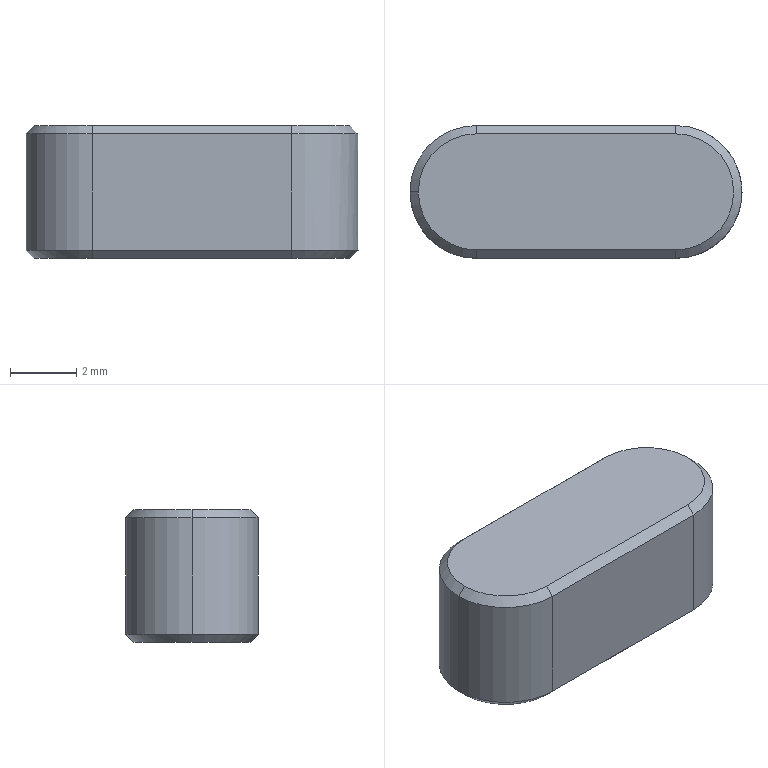Part | SolidWorks | features Boss 2, Chamfer 1, Extrusion 1 | 1 solid | 17 faces | box 10 x 4 x 4 mm | volume 144.763 mm3 | plane 8 | cone 6 | cylinder 3 | commonest cylinder face diameters 4 x3
STEP:
#1=CARTESIAN_POINT('',(-7.75,0.,2.));
#2=VERTEX_POINT('',#1);
#3=CARTESIAN_POINT('',(-6.,-1.75,2.));
#4=VERTEX_POINT('',#3);
#5=CARTESIAN_POINT('',(-6.,0.,2.));
#6=DIRECTION('',(0.,0.,1.));
#7=DIRECTION('',(-1.,0.,0.));
#8=AXIS2_PLACEMENT_3D('',#5,#6,#7);
#9=CIRCLE('',#8,1.75);
#10=EDGE_CURVE('',#2,#4,#9,.T.);
#11=ORIENTED_EDGE('',*,*,#10,.F.);
#12=CARTESIAN_POINT('',(-8.,0.,1.75));
#13=VERTEX_POINT('',#12);
#14=CARTESIAN_POINT('',(-7.75,0.,2.));
#15=DIRECTION('',(-0.7071,0.,-0.7071));
#16=VECTOR('',#15,1000.);
#17=LINE('',#14,#16);
#18=EDGE_CURVE('',#2,#13,#17,.T.);
#19=ORIENTED_EDGE('',*,*,#18,.T.);
#20=CARTESIAN_POINT('',(-6.,-2.,1.75));
#21=VERTEX_POINT('',#20);
#22=CARTESIAN_POINT('',(-6.,0.,1.75));
#23=DIRECTION('',(0.,0.,-1.));
#24=DIRECTION('',(-1.,0.,0.));
#25=AXIS2_PLACEMENT_3D('',#22,#23,#24);
#26=CIRCLE('',#25,2.);
#27=EDGE_CURVE('',#21,#13,#26,.T.);
#28=ORIENTED_EDGE('',*,*,#27,.F.);
#29=CARTESIAN_POINT('',(-6.,-1.75,2.));
#30=DIRECTION('',(0.,-0.7071,-0.7071));
#31=VECTOR('',#30,1000.);
#32=LINE('',#29,#31);
#33=EDGE_CURVE('',#4,#21,#32,.T.);
#34=ORIENTED_EDGE('',*,*,#33,.F.);
#35=EDGE_LOOP('',(#11,#19,#28,#34));
#36=FACE_OUTER_BOUND('',#35,.T.);
#37=CARTESIAN_POINT('',(-6.,0.,2.));
#38=DIRECTION('',(0.,0.,-1.));
#39=DIRECTION('',(-1.,0.,0.));
#40=AXIS2_PLACEMENT_3D('',#37,#38,#39);
#41=CONICAL_SURFACE('',#40,1.75,0.7854);
#42=ADVANCED_FACE('',(#36),#41,.T.);
#43=CARTESIAN_POINT('',(1.75,0.,-2.));
#44=VERTEX_POINT('',#43);
#45=CARTESIAN_POINT('',(0.,-1.75,-2.));
#46=VERTEX_POINT('',#45);
#47=CARTESIAN_POINT('',(0.,0.,-2.));
#48=DIRECTION('',(0.,0.,-1.));
#49=DIRECTION('',(-1.,0.,0.));
#50=AXIS2_PLACEMENT_3D('',#47,#48,#49);
#51=CIRCLE('',#50,1.75);
#52=EDGE_CURVE('',#44,#46,#51,.T.);
#53=ORIENTED_EDGE('',*,*,#52,.F.);
#54=CARTESIAN_POINT('',(2.,0.,-1.75));
#55=VERTEX_POINT('',#54);
#56=CARTESIAN_POINT('',(2.,0.,-1.75));
#57=DIRECTION('',(0.7071,0.,0.7071));
#58=VECTOR('',#57,1000.);
#59=LINE('',#56,#58);
#60=EDGE_CURVE('',#44,#55,#59,.T.);
#61=ORIENTED_EDGE('',*,*,#60,.T.);
#62=CARTESIAN_POINT('',(0.,-2.,-1.75));
#63=VERTEX_POINT('',#62);
#64=CARTESIAN_POINT('',(0.,0.,-1.75));
#65=DIRECTION('',(0.,0.,1.));
#66=DIRECTION('',(-1.,0.,0.));
#67=AXIS2_PLACEMENT_3D('',#64,#65,#66);
#68=CIRCLE('',#67,2.);
#69=EDGE_CURVE('',#63,#55,#68,.T.);
#70=ORIENTED_EDGE('',*,*,#69,.F.);
#71=CARTESIAN_POINT('',(0.,-1.75,-2.));
#72=DIRECTION('',(0.,-0.7071,0.7071));
#73=VECTOR('',#72,1000.);
#74=LINE('',#71,#73);
#75=EDGE_CURVE('',#46,#63,#74,.T.);
#76=ORIENTED_EDGE('',*,*,#75,.F.);
#77=EDGE_LOOP('',(#53,#61,#70,#76));
#78=FACE_OUTER_BOUND('',#77,.T.);
#79=CARTESIAN_POINT('',(0.,0.,-1.75));
#80=DIRECTION('',(0.,0.,1.));
#81=DIRECTION('',(1.,0.,0.));
#82=AXIS2_PLACEMENT_3D('',#79,#80,#81);
#83=CONICAL_SURFACE('',#82,2.,0.7854);
#84=ADVANCED_FACE('',(#78),#83,.T.);
#85=ORIENTED_EDGE('',*,*,#27,.T.);
#86=CARTESIAN_POINT('',(-8.,0.,-1.75));
#87=VERTEX_POINT('',#86);
#88=CARTESIAN_POINT('',(-8.,0.,2.));
#89=DIRECTION('',(0.,0.,-1.));
#90=VECTOR('',#89,1000.);
#91=LINE('',#88,#90);
#92=EDGE_CURVE('',#13,#87,#91,.T.);
#93=ORIENTED_EDGE('',*,*,#92,.T.);
#94=CARTESIAN_POINT('',(-6.,-2.,-1.75));
#95=VERTEX_POINT('',#94);
#96=CARTESIAN_POINT('',(-6.,0.,-1.75));
#97=DIRECTION('',(0.,0.,1.));
#98=DIRECTION('',(-1.,0.,0.));
#99=AXIS2_PLACEMENT_3D('',#96,#97,#98);
#100=CIRCLE('',#99,2.);
#101=EDGE_CURVE('',#87,#95,#100,.T.);
#102=ORIENTED_EDGE('',*,*,#101,.T.);
#103=CARTESIAN_POINT('',(-6.,-2.,2.));
#104=DIRECTION('',(0.,0.,-1.));
#105=VECTOR('',#104,1000.);
#106=LINE('',#103,#105);
#107=EDGE_CURVE('',#21,#95,#106,.T.);
#108=ORIENTED_EDGE('',*,*,#107,.F.);
#109=EDGE_LOOP('',(#85,#93,#102,#108));
#110=FACE_OUTER_BOUND('',#109,.T.);
#111=CARTESIAN_POINT('',(-6.,0.,2.));
#112=DIRECTION('',(0.,0.,-1.));
#113=DIRECTION('',(-1.,0.,0.));
#114=AXIS2_PLACEMENT_3D('',#111,#112,#113);
#115=CYLINDRICAL_SURFACE('',#114,2.);
#116=ADVANCED_FACE('',(#110),#115,.T.);
#117=ORIENTED_EDGE('',*,*,#92,.F.);
#118=CARTESIAN_POINT('',(-6.,2.,1.75));
#119=VERTEX_POINT('',#118);
#120=CARTESIAN_POINT('',(-6.,0.,1.75));
#121=DIRECTION('',(0.,0.,-1.));
#122=DIRECTION('',(-1.,0.,0.));
#123=AXIS2_PLACEMENT_3D('',#120,#121,#122);
#124=CIRCLE('',#123,2.);
#125=EDGE_CURVE('',#13,#119,#124,.T.);
#126=ORIENTED_EDGE('',*,*,#125,.T.);
#127=CARTESIAN_POINT('',(-6.,2.,-1.75));
#128=VERTEX_POINT('',#127);
#129=CARTESIAN_POINT('',(-6.,2.,2.));
#130=DIRECTION('',(0.,0.,-1.));
#131=VECTOR('',#130,1000.);
#132=LINE('',#129,#131);
#133=EDGE_CURVE('',#119,#128,#132,.T.);
#134=ORIENTED_EDGE('',*,*,#133,.T.);
#135=CARTESIAN_POINT('',(-6.,0.,-1.75));
#136=DIRECTION('',(0.,0.,1.));
#137=DIRECTION('',(-1.,0.,0.));
#138=AXIS2_PLACEMENT_3D('',#135,#136,#137);
#139=CIRCLE('',#138,2.);
#140=EDGE_CURVE('',#128,#87,#139,.T.);
#141=ORIENTED_EDGE('',*,*,#140,.T.);
#142=EDGE_LOOP('',(#117,#126,#134,#141));
#143=FACE_OUTER_BOUND('',#142,.T.);
#144=CARTESIAN_POINT('',(-6.,0.,2.));
#145=DIRECTION('',(0.,0.,-1.));
#146=DIRECTION('',(-1.,0.,0.));
#147=AXIS2_PLACEMENT_3D('',#144,#145,#146);
#148=CYLINDRICAL_SURFACE('',#147,2.);
#149=ADVANCED_FACE('',(#143),#148,.T.);
#150=ORIENTED_EDGE('',*,*,#107,.T.);
#151=CARTESIAN_POINT('',(0.,-2.,-1.75));
#152=DIRECTION('',(1.,0.,0.));
#153=VECTOR('',#152,1000.);
#154=LINE('',#151,#153);
#155=EDGE_CURVE('',#95,#63,#154,.T.);
#156=ORIENTED_EDGE('',*,*,#155,.T.);
#157=CARTESIAN_POINT('',(0.,-2.,1.75));
#158=VERTEX_POINT('',#157);
#159=CARTESIAN_POINT('',(0.,-2.,2.));
#160=DIRECTION('',(0.,0.,-1.));
#161=VECTOR('',#160,1000.);
#162=LINE('',#159,#161);
#163=EDGE_CURVE('',#158,#63,#162,.T.);
#164=ORIENTED_EDGE('',*,*,#163,.F.);
#165=CARTESIAN_POINT('',(0.,-2.,1.75));
#166=DIRECTION('',(-1.,0.,0.));
#167=VECTOR('',#166,1000.);
#168=LINE('',#165,#167);
#169=EDGE_CURVE('',#158,#21,#168,.T.);
#170=ORIENTED_EDGE('',*,*,#169,.T.);
#171=EDGE_LOOP('',(#150,#156,#164,#170));
#172=FACE_OUTER_BOUND('',#171,.T.);
#173=CARTESIAN_POINT('',(0.,-2.,2.));
#174=DIRECTION('',(0.,1.,0.));
#175=DIRECTION('',(0.,0.,1.));
#176=AXIS2_PLACEMENT_3D('',#173,#174,#175);
#177=PLANE('',#176);
#178=ADVANCED_FACE('',(#172),#177,.F.);
#179=CARTESIAN_POINT('',(0.,2.,1.75));
#180=VERTEX_POINT('',#179);
#181=CARTESIAN_POINT('',(0.,2.,-1.75));
#182=VERTEX_POINT('',#181);
#183=CARTESIAN_POINT('',(0.,2.,2.));
#184=DIRECTION('',(0.,0.,-1.));
#185=VECTOR('',#184,1000.);
#186=LINE('',#183,#185);
#187=EDGE_CURVE('',#180,#182,#186,.T.);
#188=ORIENTED_EDGE('',*,*,#187,.F.);
#189=CARTESIAN_POINT('',(0.,0.,1.75));
#190=DIRECTION('',(0.,0.,-1.));
#191=DIRECTION('',(-1.,0.,0.));
#192=AXIS2_PLACEMENT_3D('',#189,#190,#191);
#193=CIRCLE('',#192,2.);
#194=EDGE_CURVE('',#180,#158,#193,.T.);
#195=ORIENTED_EDGE('',*,*,#194,.T.);
#196=ORIENTED_EDGE('',*,*,#163,.T.);
#197=ORIENTED_EDGE('',*,*,#69,.T.);
#198=CARTESIAN_POINT('',(0.,0.,-1.75));
#199=DIRECTION('',(0.,0.,1.));
#200=DIRECTION('',(-1.,0.,0.));
#201=AXIS2_PLACEMENT_3D('',#198,#199,#200);
#202=CIRCLE('',#201,2.);
#203=EDGE_CURVE('',#55,#182,#202,.T.);
#204=ORIENTED_EDGE('',*,*,#203,.T.);
#205=EDGE_LOOP('',(#188,#195,#196,#197,#204));
#206=FACE_OUTER_BOUND('',#205,.T.);
#207=CARTESIAN_POINT('',(0.,0.,2.));
#208=DIRECTION('',(0.,0.,-1.));
#209=DIRECTION('',(-1.,0.,0.));
#210=AXIS2_PLACEMENT_3D('',#207,#208,#209);
#211=CYLINDRICAL_SURFACE('',#210,2.);
#212=ADVANCED_FACE('',(#206),#211,.T.);
#213=ORIENTED_EDGE('',*,*,#133,.F.);
#214=CARTESIAN_POINT('',(-6.,2.,1.75));
#215=DIRECTION('',(1.,0.,0.));
#216=VECTOR('',#215,1000.);
#217=LINE('',#214,#216);
#218=EDGE_CURVE('',#119,#180,#217,.T.);
#219=ORIENTED_EDGE('',*,*,#218,.T.);
#220=ORIENTED_EDGE('',*,*,#187,.T.);
#221=CARTESIAN_POINT('',(-6.,2.,-1.75));
#222=DIRECTION('',(-1.,0.,0.));
#223=VECTOR('',#222,1000.);
#224=LINE('',#221,#223);
#225=EDGE_CURVE('',#182,#128,#224,.T.);
#226=ORIENTED_EDGE('',*,*,#225,.T.);
#227=EDGE_LOOP('',(#213,#219,#220,#226));
#228=FACE_OUTER_BOUND('',#227,.T.);
#229=CARTESIAN_POINT('',(-6.,2.,2.));
#230=DIRECTION('',(0.,-1.,0.));
#231=DIRECTION('',(1.,0.,0.));
#232=AXIS2_PLACEMENT_3D('',#229,#230,#231);
#233=PLANE('',#232);
#234=ADVANCED_FACE('',(#228),#233,.F.);
#235=CARTESIAN_POINT('',(-6.,1.75,2.));
#236=VERTEX_POINT('',#235);
#237=CARTESIAN_POINT('',(-6.,0.,2.));
#238=DIRECTION('',(0.,0.,1.));
#239=DIRECTION('',(-1.,0.,0.));
#240=AXIS2_PLACEMENT_3D('',#237,#238,#239);
#241=CIRCLE('',#240,1.75);
#242=EDGE_CURVE('',#236,#2,#241,.T.);
#243=ORIENTED_EDGE('',*,*,#242,.T.);
#244=ORIENTED_EDGE('',*,*,#10,.T.);
#245=CARTESIAN_POINT('',(0.,-1.75,2.));
#246=VERTEX_POINT('',#245);
#247=CARTESIAN_POINT('',(-6.,-1.75,2.));
#248=DIRECTION('',(1.,0.,0.));
#249=VECTOR('',#248,1000.);
#250=LINE('',#247,#249);
#251=EDGE_CURVE('',#4,#246,#250,.T.);
#252=ORIENTED_EDGE('',*,*,#251,.T.);
#253=CARTESIAN_POINT('',(0.,1.75,2.));
#254=VERTEX_POINT('',#253);
#255=CARTESIAN_POINT('',(0.,0.,2.));
#256=DIRECTION('',(0.,0.,1.));
#257=DIRECTION('',(-1.,0.,0.));
#258=AXIS2_PLACEMENT_3D('',#255,#256,#257);
#259=CIRCLE('',#258,1.75);
#260=EDGE_CURVE('',#246,#254,#259,.T.);
#261=ORIENTED_EDGE('',*,*,#260,.T.);
#262=CARTESIAN_POINT('',(-6.,1.75,2.));
#263=DIRECTION('',(-1.,0.,0.));
#264=VECTOR('',#263,1000.);
#265=LINE('',#262,#264);
#266=EDGE_CURVE('',#254,#236,#265,.T.);
#267=ORIENTED_EDGE('',*,*,#266,.T.);
#268=EDGE_LOOP('',(#243,#244,#252,#261,#267));
#269=FACE_OUTER_BOUND('',#268,.T.);
#270=CARTESIAN_POINT('',(-6.,0.,2.));
#271=DIRECTION('',(0.,0.,-1.));
#272=DIRECTION('',(-1.,0.,0.));
#273=AXIS2_PLACEMENT_3D('',#270,#271,#272);
#274=PLANE('',#273);
#275=ADVANCED_FACE('',(#269),#274,.F.);
#276=CARTESIAN_POINT('',(0.,1.75,-2.));
#277=VERTEX_POINT('',#276);
#278=CARTESIAN_POINT('',(0.,0.,-2.));
#279=DIRECTION('',(0.,0.,-1.));
#280=DIRECTION('',(-1.,0.,0.));
#281=AXIS2_PLACEMENT_3D('',#278,#279,#280);
#282=CIRCLE('',#281,1.75);
#283=EDGE_CURVE('',#277,#44,#282,.T.);
#284=ORIENTED_EDGE('',*,*,#283,.T.);
#285=ORIENTED_EDGE('',*,*,#52,.T.);
#286=CARTESIAN_POINT('',(-6.,-1.75,-2.));
#287=VERTEX_POINT('',#286);
#288=CARTESIAN_POINT('',(-6.,-1.75,-2.));
#289=DIRECTION('',(-1.,0.,0.));
#290=VECTOR('',#289,1000.);
#291=LINE('',#288,#290);
#292=EDGE_CURVE('',#46,#287,#291,.T.);
#293=ORIENTED_EDGE('',*,*,#292,.T.);
#294=CARTESIAN_POINT('',(-6.,1.75,-2.));
#295=VERTEX_POINT('',#294);
#296=CARTESIAN_POINT('',(-6.,0.,-2.));
#297=DIRECTION('',(0.,0.,-1.));
#298=DIRECTION('',(-1.,0.,0.));
#299=AXIS2_PLACEMENT_3D('',#296,#297,#298);
#300=CIRCLE('',#299,1.75);
#301=EDGE_CURVE('',#287,#295,#300,.T.);
#302=ORIENTED_EDGE('',*,*,#301,.T.);
#303=CARTESIAN_POINT('',(0.,1.75,-2.));
#304=DIRECTION('',(1.,0.,0.));
#305=VECTOR('',#304,1000.);
#306=LINE('',#303,#305);
#307=EDGE_CURVE('',#295,#277,#306,.T.);
#308=ORIENTED_EDGE('',*,*,#307,.T.);
#309=EDGE_LOOP('',(#284,#285,#293,#302,#308));
#310=FACE_OUTER_BOUND('',#309,.T.);
#311=CARTESIAN_POINT('',(-6.,0.,-2.));
#312=DIRECTION('',(0.,0.,-1.));
#313=DIRECTION('',(-1.,0.,0.));
#314=AXIS2_PLACEMENT_3D('',#311,#312,#313);
#315=PLANE('',#314);
#316=ADVANCED_FACE('',(#310),#315,.T.);
#317=CARTESIAN_POINT('',(0.,1.75,-2.));
#318=DIRECTION('',(0.,0.7071,0.7071));
#319=VECTOR('',#318,1000.);
#320=LINE('',#317,#319);
#321=EDGE_CURVE('',#277,#182,#320,.T.);
#322=ORIENTED_EDGE('',*,*,#321,.F.);
#323=ORIENTED_EDGE('',*,*,#307,.F.);
#324=CARTESIAN_POINT('',(-6.,2.,-1.75));
#325=DIRECTION('',(0.,-0.7071,-0.7071));
#326=VECTOR('',#325,1000.);
#327=LINE('',#324,#326);
#328=EDGE_CURVE('',#128,#295,#327,.T.);
#329=ORIENTED_EDGE('',*,*,#328,.F.);
#330=ORIENTED_EDGE('',*,*,#225,.F.);
#331=EDGE_LOOP('',(#322,#323,#329,#330));
#332=FACE_OUTER_BOUND('',#331,.T.);
#333=CARTESIAN_POINT('',(-6.,2.,-1.75));
#334=DIRECTION('',(0.,0.7071,-0.7071));
#335=DIRECTION('',(0.,0.7071,0.7071));
#336=AXIS2_PLACEMENT_3D('',#333,#334,#335);
#337=PLANE('',#336);
#338=ADVANCED_FACE('',(#332),#337,.T.);
#339=ORIENTED_EDGE('',*,*,#328,.T.);
#340=ORIENTED_EDGE('',*,*,#301,.F.);
#341=CARTESIAN_POINT('',(-6.,-2.,-1.75));
#342=DIRECTION('',(0.,0.7071,-0.7071));
#343=VECTOR('',#342,1000.);
#344=LINE('',#341,#343);
#345=EDGE_CURVE('',#95,#287,#344,.T.);
#346=ORIENTED_EDGE('',*,*,#345,.F.);
#347=ORIENTED_EDGE('',*,*,#101,.F.);
#348=ORIENTED_EDGE('',*,*,#140,.F.);
#349=EDGE_LOOP('',(#339,#340,#346,#347,#348));
#350=FACE_OUTER_BOUND('',#349,.T.);
#351=CARTESIAN_POINT('',(-6.,0.,-1.75));
#352=DIRECTION('',(0.,0.,1.));
#353=DIRECTION('',(1.,0.,0.));
#354=AXIS2_PLACEMENT_3D('',#351,#352,#353);
#355=CONICAL_SURFACE('',#354,2.,0.7854);
#356=ADVANCED_FACE('',(#350),#355,.T.);
#357=ORIENTED_EDGE('',*,*,#60,.F.);
#358=ORIENTED_EDGE('',*,*,#283,.F.);
#359=ORIENTED_EDGE('',*,*,#321,.T.);
#360=ORIENTED_EDGE('',*,*,#203,.F.);
#361=EDGE_LOOP('',(#357,#358,#359,#360));
#362=FACE_OUTER_BOUND('',#361,.T.);
#363=CARTESIAN_POINT('',(0.,0.,-1.75));
#364=DIRECTION('',(0.,0.,1.));
#365=DIRECTION('',(1.,0.,0.));
#366=AXIS2_PLACEMENT_3D('',#363,#364,#365);
#367=CONICAL_SURFACE('',#366,2.,0.7854);
#368=ADVANCED_FACE('',(#362),#367,.T.);
#369=ORIENTED_EDGE('',*,*,#345,.T.);
#370=ORIENTED_EDGE('',*,*,#292,.F.);
#371=ORIENTED_EDGE('',*,*,#75,.T.);
#372=ORIENTED_EDGE('',*,*,#155,.F.);
#373=EDGE_LOOP('',(#369,#370,#371,#372));
#374=FACE_OUTER_BOUND('',#373,.T.);
#375=CARTESIAN_POINT('',(0.,-2.,-1.75));
#376=DIRECTION('',(0.,-0.7071,-0.7071));
#377=DIRECTION('',(0.,0.7071,-0.7071));
#378=AXIS2_PLACEMENT_3D('',#375,#376,#377);
#379=PLANE('',#378);
#380=ADVANCED_FACE('',(#374),#379,.T.);
#381=CARTESIAN_POINT('',(0.,2.,1.75));
#382=DIRECTION('',(0.,-0.7071,0.7071));
#383=VECTOR('',#382,1000.);
#384=LINE('',#381,#383);
#385=EDGE_CURVE('',#180,#254,#384,.T.);
#386=ORIENTED_EDGE('',*,*,#385,.F.);
#387=ORIENTED_EDGE('',*,*,#218,.F.);
#388=CARTESIAN_POINT('',(-6.,1.75,2.));
#389=DIRECTION('',(0.,0.7071,-0.7071));
#390=VECTOR('',#389,1000.);
#391=LINE('',#388,#390);
#392=EDGE_CURVE('',#236,#119,#391,.T.);
#393=ORIENTED_EDGE('',*,*,#392,.F.);
#394=ORIENTED_EDGE('',*,*,#266,.F.);
#395=EDGE_LOOP('',(#386,#387,#393,#394));
#396=FACE_OUTER_BOUND('',#395,.T.);
#397=CARTESIAN_POINT('',(-6.,1.75,2.));
#398=DIRECTION('',(0.,-0.7071,-0.7071));
#399=DIRECTION('',(0.,0.7071,-0.7071));
#400=AXIS2_PLACEMENT_3D('',#397,#398,#399);
#401=PLANE('',#400);
#402=ADVANCED_FACE('',(#396),#401,.F.);
#403=ORIENTED_EDGE('',*,*,#18,.F.);
#404=ORIENTED_EDGE('',*,*,#242,.F.);
#405=ORIENTED_EDGE('',*,*,#392,.T.);
#406=ORIENTED_EDGE('',*,*,#125,.F.);
#407=EDGE_LOOP('',(#403,#404,#405,#406));
#408=FACE_OUTER_BOUND('',#407,.T.);
#409=CARTESIAN_POINT('',(-6.,0.,2.));
#410=DIRECTION('',(0.,0.,-1.));
#411=DIRECTION('',(-1.,0.,0.));
#412=AXIS2_PLACEMENT_3D('',#409,#410,#411);
#413=CONICAL_SURFACE('',#412,1.75,0.7854);
#414=ADVANCED_FACE('',(#408),#413,.T.);
#415=ORIENTED_EDGE('',*,*,#385,.T.);
#416=ORIENTED_EDGE('',*,*,#260,.F.);
#417=CARTESIAN_POINT('',(0.,-2.,1.75));
#418=DIRECTION('',(0.,0.7071,0.7071));
#419=VECTOR('',#418,1000.);
#420=LINE('',#417,#419);
#421=EDGE_CURVE('',#158,#246,#420,.T.);
#422=ORIENTED_EDGE('',*,*,#421,.F.);
#423=ORIENTED_EDGE('',*,*,#194,.F.);
#424=EDGE_LOOP('',(#415,#416,#422,#423));
#425=FACE_OUTER_BOUND('',#424,.T.);
#426=CARTESIAN_POINT('',(0.,0.,2.));
#427=DIRECTION('',(0.,0.,-1.));
#428=DIRECTION('',(-1.,0.,0.));
#429=AXIS2_PLACEMENT_3D('',#426,#427,#428);
#430=CONICAL_SURFACE('',#429,1.75,0.7854);
#431=ADVANCED_FACE('',(#425),#430,.T.);
#432=ORIENTED_EDGE('',*,*,#33,.T.);
#433=ORIENTED_EDGE('',*,*,#169,.F.);
#434=ORIENTED_EDGE('',*,*,#421,.T.);
#435=ORIENTED_EDGE('',*,*,#251,.F.);
#436=EDGE_LOOP('',(#432,#433,#434,#435));
#437=FACE_OUTER_BOUND('',#436,.T.);
#438=CARTESIAN_POINT('',(-6.,-1.75,2.));
#439=DIRECTION('',(0.,0.7071,-0.7071));
#440=DIRECTION('',(0.,0.7071,0.7071));
#441=AXIS2_PLACEMENT_3D('',#438,#439,#440);
#442=PLANE('',#441);
#443=ADVANCED_FACE('',(#437),#442,.F.);
#444=CLOSED_SHELL('',(#42,#84,#116,#149,#178,#212,#234,#275,#316,#338,#356,#368,#380,#402,#414,#431,#443));
#445=MANIFOLD_SOLID_BREP('',#444);
#446=CARTESIAN_POINT('',(0.,0.,0.));
#447=DIRECTION('',(0.,0.,1.));
#448=DIRECTION('',(1.,0.,0.));
#449=AXIS2_PLACEMENT_3D('',#446,#447,#448);
#450=(LENGTH_UNIT()NAMED_UNIT(*)SI_UNIT(.MILLI.,.METRE.));
#451=UNCERTAINTY_MEASURE_WITH_UNIT(LENGTH_MEASURE(0.00001),#450,'','');
#452=(NAMED_UNIT(*)PLANE_ANGLE_UNIT()SI_UNIT($,.RADIAN.));
#453=(NAMED_UNIT(*)SI_UNIT($,.STERADIAN.)SOLID_ANGLE_UNIT());
#454=(GEOMETRIC_REPRESENTATION_CONTEXT(3)GLOBAL_UNCERTAINTY_ASSIGNED_CONTEXT((#451))GLOBAL_UNIT_ASSIGNED_CONTEXT((#450,#452,#453))REPRESENTATION_CONTEXT('',''));
#455=ADVANCED_BREP_SHAPE_REPRESENTATION('',(#445,#449),#454);